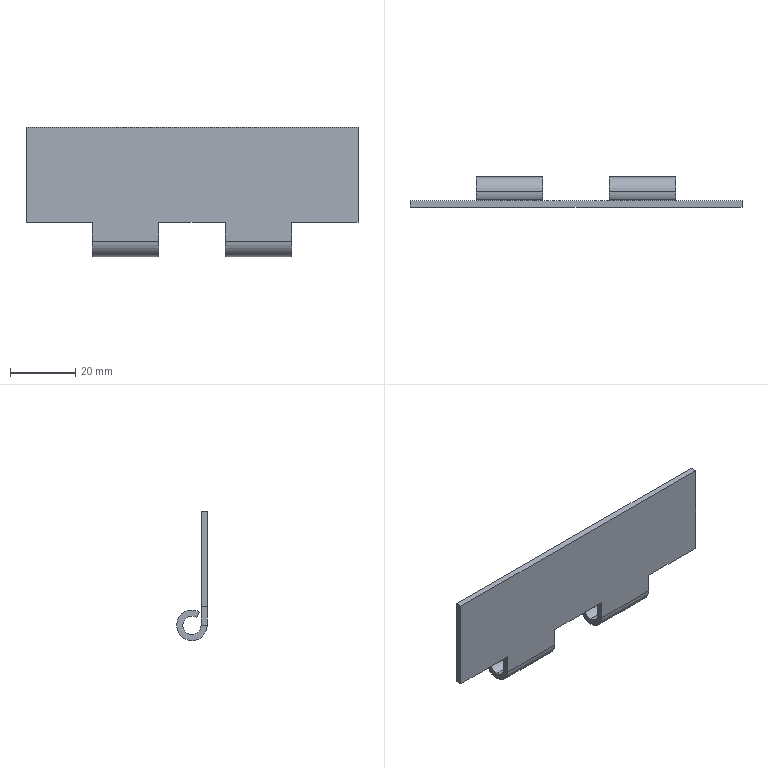Part | SolidWorks | features FlatPattern 1, ICE 1, SMBaseFlange 1, SheetMetal 1 | 1 solid | 28 faces | box 102 x 9.4 x 39.7 mm | volume 7631 mm3 | plane 16 | cylinder 12 | commonest cylinder face diameters 5.6 x6 9.4 x6
STEP:
#1=CARTESIAN_POINT('',(30.6,4.7,-37.8));
#2=VERTEX_POINT('',#1);
#3=CARTESIAN_POINT('',(30.6,1.9,-35.));
#4=VERTEX_POINT('',#3);
#5=CARTESIAN_POINT('',(30.6,4.7,-35.));
#6=DIRECTION('',(-1.,0.,0.));
#7=DIRECTION('',(0.,0.,1.));
#8=AXIS2_PLACEMENT_3D('',#5,#6,#7);
#9=CIRCLE('',#8,2.8);
#10=EDGE_CURVE('',#2,#4,#9,.T.);
#11=ORIENTED_EDGE('',*,*,#10,.F.);
#12=CARTESIAN_POINT('',(10.2,4.7,-37.8));
#13=VERTEX_POINT('',#12);
#14=CARTESIAN_POINT('',(51.,4.7,-37.8));
#15=DIRECTION('',(-1.,0.,0.));
#16=VECTOR('',#15,1000.);
#17=LINE('',#14,#16);
#18=EDGE_CURVE('',#2,#13,#17,.T.);
#19=ORIENTED_EDGE('',*,*,#18,.T.);
#20=CARTESIAN_POINT('',(10.2,1.9,-35.));
#21=VERTEX_POINT('',#20);
#22=CARTESIAN_POINT('',(10.2,4.7,-35.));
#23=DIRECTION('',(1.,0.,0.));
#24=DIRECTION('',(0.,0.,-1.));
#25=AXIS2_PLACEMENT_3D('',#22,#23,#24);
#26=CIRCLE('',#25,2.8);
#27=EDGE_CURVE('',#21,#13,#26,.T.);
#28=ORIENTED_EDGE('',*,*,#27,.F.);
#29=CARTESIAN_POINT('',(51.,1.9,-35.));
#30=DIRECTION('',(-1.,0.,0.));
#31=VECTOR('',#30,1000.);
#32=LINE('',#29,#31);
#33=EDGE_CURVE('',#4,#21,#32,.T.);
#34=ORIENTED_EDGE('',*,*,#33,.F.);
#35=EDGE_LOOP('',(#11,#19,#28,#34));
#36=FACE_OUTER_BOUND('',#35,.T.);
#37=CARTESIAN_POINT('',(51.,4.7,-35.));
#38=DIRECTION('',(-1.,0.,0.));
#39=DIRECTION('',(0.,0.,1.));
#40=AXIS2_PLACEMENT_3D('',#37,#38,#39);
#41=CYLINDRICAL_SURFACE('',#40,2.8);
#42=ADVANCED_FACE('',(#36),#41,.F.);
#43=ORIENTED_EDGE('',*,*,#18,.F.);
#44=CARTESIAN_POINT('',(30.6,4.7,-32.2));
#45=VERTEX_POINT('',#44);
#46=CARTESIAN_POINT('',(30.6,4.7,-35.));
#47=DIRECTION('',(-1.,0.,0.));
#48=DIRECTION('',(0.,0.,1.));
#49=AXIS2_PLACEMENT_3D('',#46,#47,#48);
#50=CIRCLE('',#49,2.8);
#51=EDGE_CURVE('',#45,#2,#50,.T.);
#52=ORIENTED_EDGE('',*,*,#51,.F.);
#53=CARTESIAN_POINT('',(10.2,4.7,-32.2));
#54=VERTEX_POINT('',#53);
#55=CARTESIAN_POINT('',(51.,4.7,-32.2));
#56=DIRECTION('',(-1.,0.,0.));
#57=VECTOR('',#56,1000.);
#58=LINE('',#55,#57);
#59=EDGE_CURVE('',#45,#54,#58,.T.);
#60=ORIENTED_EDGE('',*,*,#59,.T.);
#61=CARTESIAN_POINT('',(10.2,4.7,-35.));
#62=DIRECTION('',(1.,0.,0.));
#63=DIRECTION('',(0.,0.,-1.));
#64=AXIS2_PLACEMENT_3D('',#61,#62,#63);
#65=CIRCLE('',#64,2.8);
#66=EDGE_CURVE('',#13,#54,#65,.T.);
#67=ORIENTED_EDGE('',*,*,#66,.F.);
#68=EDGE_LOOP('',(#43,#52,#60,#67));
#69=FACE_OUTER_BOUND('',#68,.T.);
#70=CARTESIAN_POINT('',(51.,4.7,-35.));
#71=DIRECTION('',(-1.,0.,0.));
#72=DIRECTION('',(0.,0.,1.));
#73=AXIS2_PLACEMENT_3D('',#70,#71,#72);
#74=CYLINDRICAL_SURFACE('',#73,2.8);
#75=ADVANCED_FACE('',(#69),#74,.F.);
#76=CARTESIAN_POINT('',(30.6,4.7,-30.3));
#77=VERTEX_POINT('',#76);
#78=CARTESIAN_POINT('',(30.6,4.7,-39.7));
#79=VERTEX_POINT('',#78);
#80=CARTESIAN_POINT('',(30.6,4.7,-35.));
#81=DIRECTION('',(-1.,0.,0.));
#82=DIRECTION('',(0.,0.,1.));
#83=AXIS2_PLACEMENT_3D('',#80,#81,#82);
#84=CIRCLE('',#83,4.7);
#85=EDGE_CURVE('',#77,#79,#84,.T.);
#86=ORIENTED_EDGE('',*,*,#85,.T.);
#87=CARTESIAN_POINT('',(10.2,4.7,-39.7));
#88=VERTEX_POINT('',#87);
#89=CARTESIAN_POINT('',(51.,4.7,-39.7));
#90=DIRECTION('',(-1.,0.,0.));
#91=VECTOR('',#90,1000.);
#92=LINE('',#89,#91);
#93=EDGE_CURVE('',#79,#88,#92,.T.);
#94=ORIENTED_EDGE('',*,*,#93,.T.);
#95=CARTESIAN_POINT('',(10.2,4.7,-30.3));
#96=VERTEX_POINT('',#95);
#97=CARTESIAN_POINT('',(10.2,4.7,-35.));
#98=DIRECTION('',(1.,0.,0.));
#99=DIRECTION('',(0.,0.,-1.));
#100=AXIS2_PLACEMENT_3D('',#97,#98,#99);
#101=CIRCLE('',#100,4.7);
#102=EDGE_CURVE('',#88,#96,#101,.T.);
#103=ORIENTED_EDGE('',*,*,#102,.T.);
#104=CARTESIAN_POINT('',(51.,4.7,-30.3));
#105=DIRECTION('',(-1.,0.,0.));
#106=VECTOR('',#105,1000.);
#107=LINE('',#104,#106);
#108=EDGE_CURVE('',#77,#96,#107,.T.);
#109=ORIENTED_EDGE('',*,*,#108,.F.);
#110=EDGE_LOOP('',(#86,#94,#103,#109));
#111=FACE_OUTER_BOUND('',#110,.T.);
#112=CARTESIAN_POINT('',(51.,4.7,-35.));
#113=DIRECTION('',(-1.,0.,0.));
#114=DIRECTION('',(0.,0.,1.));
#115=AXIS2_PLACEMENT_3D('',#112,#113,#114);
#116=CYLINDRICAL_SURFACE('',#115,4.7);
#117=ADVANCED_FACE('',(#111),#116,.T.);
#118=CARTESIAN_POINT('',(30.6,2.35,-30.93));
#119=VERTEX_POINT('',#118);
#120=CARTESIAN_POINT('',(30.6,4.7,-35.));
#121=DIRECTION('',(-1.,0.,0.));
#122=DIRECTION('',(0.,0.,1.));
#123=AXIS2_PLACEMENT_3D('',#120,#121,#122);
#124=CIRCLE('',#123,4.7);
#125=EDGE_CURVE('',#119,#77,#124,.T.);
#126=ORIENTED_EDGE('',*,*,#125,.T.);
#127=ORIENTED_EDGE('',*,*,#108,.T.);
#128=CARTESIAN_POINT('',(10.2,2.35,-30.93));
#129=VERTEX_POINT('',#128);
#130=CARTESIAN_POINT('',(10.2,4.7,-35.));
#131=DIRECTION('',(1.,0.,0.));
#132=DIRECTION('',(0.,0.,-1.));
#133=AXIS2_PLACEMENT_3D('',#130,#131,#132);
#134=CIRCLE('',#133,4.7);
#135=EDGE_CURVE('',#96,#129,#134,.T.);
#136=ORIENTED_EDGE('',*,*,#135,.T.);
#137=CARTESIAN_POINT('',(51.,2.35,-30.93));
#138=DIRECTION('',(-1.,0.,0.));
#139=VECTOR('',#138,1000.);
#140=LINE('',#137,#139);
#141=EDGE_CURVE('',#119,#129,#140,.T.);
#142=ORIENTED_EDGE('',*,*,#141,.F.);
#143=EDGE_LOOP('',(#126,#127,#136,#142));
#144=FACE_OUTER_BOUND('',#143,.T.);
#145=CARTESIAN_POINT('',(51.,4.7,-35.));
#146=DIRECTION('',(-1.,0.,0.));
#147=DIRECTION('',(0.,0.,1.));
#148=AXIS2_PLACEMENT_3D('',#145,#146,#147);
#149=CYLINDRICAL_SURFACE('',#148,4.7);
#150=ADVANCED_FACE('',(#144),#149,.T.);
#151=CARTESIAN_POINT('',(-10.2,4.7,-37.8));
#152=VERTEX_POINT('',#151);
#153=CARTESIAN_POINT('',(-10.2,1.9,-35.));
#154=VERTEX_POINT('',#153);
#155=CARTESIAN_POINT('',(-10.2,4.7,-35.));
#156=DIRECTION('',(-1.,0.,0.));
#157=DIRECTION('',(0.,0.,1.));
#158=AXIS2_PLACEMENT_3D('',#155,#156,#157);
#159=CIRCLE('',#158,2.8);
#160=EDGE_CURVE('',#152,#154,#159,.T.);
#161=ORIENTED_EDGE('',*,*,#160,.F.);
#162=CARTESIAN_POINT('',(-30.6,4.7,-37.8));
#163=VERTEX_POINT('',#162);
#164=CARTESIAN_POINT('',(51.,4.7,-37.8));
#165=DIRECTION('',(-1.,0.,0.));
#166=VECTOR('',#165,1000.);
#167=LINE('',#164,#166);
#168=EDGE_CURVE('',#152,#163,#167,.T.);
#169=ORIENTED_EDGE('',*,*,#168,.T.);
#170=CARTESIAN_POINT('',(-30.6,1.9,-35.));
#171=VERTEX_POINT('',#170);
#172=CARTESIAN_POINT('',(-30.6,4.7,-35.));
#173=DIRECTION('',(1.,0.,0.));
#174=DIRECTION('',(0.,0.,-1.));
#175=AXIS2_PLACEMENT_3D('',#172,#173,#174);
#176=CIRCLE('',#175,2.8);
#177=EDGE_CURVE('',#171,#163,#176,.T.);
#178=ORIENTED_EDGE('',*,*,#177,.F.);
#179=CARTESIAN_POINT('',(51.,1.9,-35.));
#180=DIRECTION('',(-1.,0.,0.));
#181=VECTOR('',#180,1000.);
#182=LINE('',#179,#181);
#183=EDGE_CURVE('',#154,#171,#182,.T.);
#184=ORIENTED_EDGE('',*,*,#183,.F.);
#185=EDGE_LOOP('',(#161,#169,#178,#184));
#186=FACE_OUTER_BOUND('',#185,.T.);
#187=CARTESIAN_POINT('',(51.,4.7,-35.));
#188=DIRECTION('',(-1.,0.,0.));
#189=DIRECTION('',(0.,0.,1.));
#190=AXIS2_PLACEMENT_3D('',#187,#188,#189);
#191=CYLINDRICAL_SURFACE('',#190,2.8);
#192=ADVANCED_FACE('',(#186),#191,.F.);
#193=ORIENTED_EDGE('',*,*,#168,.F.);
#194=CARTESIAN_POINT('',(-10.2,4.7,-32.2));
#195=VERTEX_POINT('',#194);
#196=CARTESIAN_POINT('',(-10.2,4.7,-35.));
#197=DIRECTION('',(-1.,0.,0.));
#198=DIRECTION('',(0.,0.,1.));
#199=AXIS2_PLACEMENT_3D('',#196,#197,#198);
#200=CIRCLE('',#199,2.8);
#201=EDGE_CURVE('',#195,#152,#200,.T.);
#202=ORIENTED_EDGE('',*,*,#201,.F.);
#203=CARTESIAN_POINT('',(-30.6,4.7,-32.2));
#204=VERTEX_POINT('',#203);
#205=CARTESIAN_POINT('',(51.,4.7,-32.2));
#206=DIRECTION('',(-1.,0.,0.));
#207=VECTOR('',#206,1000.);
#208=LINE('',#205,#207);
#209=EDGE_CURVE('',#195,#204,#208,.T.);
#210=ORIENTED_EDGE('',*,*,#209,.T.);
#211=CARTESIAN_POINT('',(-30.6,4.7,-35.));
#212=DIRECTION('',(1.,0.,0.));
#213=DIRECTION('',(0.,0.,-1.));
#214=AXIS2_PLACEMENT_3D('',#211,#212,#213);
#215=CIRCLE('',#214,2.8);
#216=EDGE_CURVE('',#163,#204,#215,.T.);
#217=ORIENTED_EDGE('',*,*,#216,.F.);
#218=EDGE_LOOP('',(#193,#202,#210,#217));
#219=FACE_OUTER_BOUND('',#218,.T.);
#220=CARTESIAN_POINT('',(51.,4.7,-35.));
#221=DIRECTION('',(-1.,0.,0.));
#222=DIRECTION('',(0.,0.,1.));
#223=AXIS2_PLACEMENT_3D('',#220,#221,#222);
#224=CYLINDRICAL_SURFACE('',#223,2.8);
#225=ADVANCED_FACE('',(#219),#224,.F.);
#226=CARTESIAN_POINT('',(-10.2,4.7,-30.3));
#227=VERTEX_POINT('',#226);
#228=CARTESIAN_POINT('',(-10.2,4.7,-39.7));
#229=VERTEX_POINT('',#228);
#230=CARTESIAN_POINT('',(-10.2,4.7,-35.));
#231=DIRECTION('',(-1.,0.,0.));
#232=DIRECTION('',(0.,0.,1.));
#233=AXIS2_PLACEMENT_3D('',#230,#231,#232);
#234=CIRCLE('',#233,4.7);
#235=EDGE_CURVE('',#227,#229,#234,.T.);
#236=ORIENTED_EDGE('',*,*,#235,.T.);
#237=CARTESIAN_POINT('',(-30.6,4.7,-39.7));
#238=VERTEX_POINT('',#237);
#239=CARTESIAN_POINT('',(51.,4.7,-39.7));
#240=DIRECTION('',(-1.,0.,0.));
#241=VECTOR('',#240,1000.);
#242=LINE('',#239,#241);
#243=EDGE_CURVE('',#229,#238,#242,.T.);
#244=ORIENTED_EDGE('',*,*,#243,.T.);
#245=CARTESIAN_POINT('',(-30.6,4.7,-30.3));
#246=VERTEX_POINT('',#245);
#247=CARTESIAN_POINT('',(-30.6,4.7,-35.));
#248=DIRECTION('',(1.,0.,0.));
#249=DIRECTION('',(0.,0.,-1.));
#250=AXIS2_PLACEMENT_3D('',#247,#248,#249);
#251=CIRCLE('',#250,4.7);
#252=EDGE_CURVE('',#238,#246,#251,.T.);
#253=ORIENTED_EDGE('',*,*,#252,.T.);
#254=CARTESIAN_POINT('',(51.,4.7,-30.3));
#255=DIRECTION('',(-1.,0.,0.));
#256=VECTOR('',#255,1000.);
#257=LINE('',#254,#256);
#258=EDGE_CURVE('',#227,#246,#257,.T.);
#259=ORIENTED_EDGE('',*,*,#258,.F.);
#260=EDGE_LOOP('',(#236,#244,#253,#259));
#261=FACE_OUTER_BOUND('',#260,.T.);
#262=CARTESIAN_POINT('',(51.,4.7,-35.));
#263=DIRECTION('',(-1.,0.,0.));
#264=DIRECTION('',(0.,0.,1.));
#265=AXIS2_PLACEMENT_3D('',#262,#263,#264);
#266=CYLINDRICAL_SURFACE('',#265,4.7);
#267=ADVANCED_FACE('',(#261),#266,.T.);
#268=CARTESIAN_POINT('',(-10.2,2.35,-30.93));
#269=VERTEX_POINT('',#268);
#270=CARTESIAN_POINT('',(-10.2,4.7,-35.));
#271=DIRECTION('',(-1.,0.,0.));
#272=DIRECTION('',(0.,0.,1.));
#273=AXIS2_PLACEMENT_3D('',#270,#271,#272);
#274=CIRCLE('',#273,4.7);
#275=EDGE_CURVE('',#269,#227,#274,.T.);
#276=ORIENTED_EDGE('',*,*,#275,.T.);
#277=ORIENTED_EDGE('',*,*,#258,.T.);
#278=CARTESIAN_POINT('',(-30.6,2.35,-30.93));
#279=VERTEX_POINT('',#278);
#280=CARTESIAN_POINT('',(-30.6,4.7,-35.));
#281=DIRECTION('',(1.,0.,0.));
#282=DIRECTION('',(0.,0.,-1.));
#283=AXIS2_PLACEMENT_3D('',#280,#281,#282);
#284=CIRCLE('',#283,4.7);
#285=EDGE_CURVE('',#246,#279,#284,.T.);
#286=ORIENTED_EDGE('',*,*,#285,.T.);
#287=CARTESIAN_POINT('',(51.,2.35,-30.93));
#288=DIRECTION('',(-1.,0.,0.));
#289=VECTOR('',#288,1000.);
#290=LINE('',#287,#289);
#291=EDGE_CURVE('',#269,#279,#290,.T.);
#292=ORIENTED_EDGE('',*,*,#291,.F.);
#293=EDGE_LOOP('',(#276,#277,#286,#292));
#294=FACE_OUTER_BOUND('',#293,.T.);
#295=CARTESIAN_POINT('',(51.,4.7,-35.));
#296=DIRECTION('',(-1.,0.,0.));
#297=DIRECTION('',(0.,0.,1.));
#298=AXIS2_PLACEMENT_3D('',#295,#296,#297);
#299=CYLINDRICAL_SURFACE('',#298,4.7);
#300=ADVANCED_FACE('',(#294),#299,.T.);
#301=CARTESIAN_POINT('',(10.2,1.9,-29.2));
#302=VERTEX_POINT('',#301);
#303=CARTESIAN_POINT('',(10.2,1.9,0.));
#304=DIRECTION('',(0.,0.,-1.));
#305=VECTOR('',#304,1000.);
#306=LINE('',#303,#305);
#307=EDGE_CURVE('',#302,#21,#306,.T.);
#308=ORIENTED_EDGE('',*,*,#307,.T.);
#309=CARTESIAN_POINT('',(10.2,0.,-35.));
#310=VERTEX_POINT('',#309);
#311=CARTESIAN_POINT('',(10.2,1.9,-35.));
#312=DIRECTION('',(0.,-1.,0.));
#313=VECTOR('',#312,1000.);
#314=LINE('',#311,#313);
#315=EDGE_CURVE('',#21,#310,#314,.T.);
#316=ORIENTED_EDGE('',*,*,#315,.T.);
#317=CARTESIAN_POINT('',(10.2,0.,-29.2));
#318=VERTEX_POINT('',#317);
#319=CARTESIAN_POINT('',(10.2,0.,0.));
#320=DIRECTION('',(0.,0.,-1.));
#321=VECTOR('',#320,1000.);
#322=LINE('',#319,#321);
#323=EDGE_CURVE('',#318,#310,#322,.T.);
#324=ORIENTED_EDGE('',*,*,#323,.F.);
#325=CARTESIAN_POINT('',(10.2,9.4,-29.2));
#326=DIRECTION('',(0.,-1.,0.));
#327=VECTOR('',#326,1000.);
#328=LINE('',#325,#327);
#329=EDGE_CURVE('',#302,#318,#328,.T.);
#330=ORIENTED_EDGE('',*,*,#329,.F.);
#331=EDGE_LOOP('',(#308,#316,#324,#330));
#332=FACE_OUTER_BOUND('',#331,.T.);
#333=CARTESIAN_POINT('',(10.2,9.4,-39.7));
#334=DIRECTION('',(1.,0.,0.));
#335=DIRECTION('',(0.,0.,-1.));
#336=AXIS2_PLACEMENT_3D('',#333,#334,#335);
#337=PLANE('',#336);
#338=ADVANCED_FACE('',(#332),#337,.F.);
#339=CARTESIAN_POINT('',(-30.6,1.9,-29.2));
#340=VERTEX_POINT('',#339);
#341=CARTESIAN_POINT('',(-30.6,1.9,0.));
#342=DIRECTION('',(0.,0.,-1.));
#343=VECTOR('',#342,1000.);
#344=LINE('',#341,#343);
#345=EDGE_CURVE('',#340,#171,#344,.T.);
#346=ORIENTED_EDGE('',*,*,#345,.T.);
#347=CARTESIAN_POINT('',(-30.6,0.,-35.));
#348=VERTEX_POINT('',#347);
#349=CARTESIAN_POINT('',(-30.6,1.9,-35.));
#350=DIRECTION('',(0.,-1.,0.));
#351=VECTOR('',#350,1000.);
#352=LINE('',#349,#351);
#353=EDGE_CURVE('',#171,#348,#352,.T.);
#354=ORIENTED_EDGE('',*,*,#353,.T.);
#355=CARTESIAN_POINT('',(-30.6,0.,-29.2));
#356=VERTEX_POINT('',#355);
#357=CARTESIAN_POINT('',(-30.6,0.,-39.7));
#358=DIRECTION('',(0.,0.,1.));
#359=VECTOR('',#358,1000.);
#360=LINE('',#357,#359);
#361=EDGE_CURVE('',#348,#356,#360,.T.);
#362=ORIENTED_EDGE('',*,*,#361,.T.);
#363=CARTESIAN_POINT('',(-30.6,9.4,-29.2));
#364=DIRECTION('',(0.,-1.,0.));
#365=VECTOR('',#364,1000.);
#366=LINE('',#363,#365);
#367=EDGE_CURVE('',#340,#356,#366,.T.);
#368=ORIENTED_EDGE('',*,*,#367,.F.);
#369=EDGE_LOOP('',(#346,#354,#362,#368));
#370=FACE_OUTER_BOUND('',#369,.T.);
#371=CARTESIAN_POINT('',(-30.6,9.4,-39.7));
#372=DIRECTION('',(1.,0.,0.));
#373=DIRECTION('',(0.,0.,-1.));
#374=AXIS2_PLACEMENT_3D('',#371,#372,#373);
#375=PLANE('',#374);
#376=ADVANCED_FACE('',(#370),#375,.F.);
#377=ORIENTED_EDGE('',*,*,#243,.F.);
#378=CARTESIAN_POINT('',(-10.2,0.,-35.));
#379=VERTEX_POINT('',#378);
#380=CARTESIAN_POINT('',(-10.2,4.7,-35.));
#381=DIRECTION('',(-1.,0.,0.));
#382=DIRECTION('',(0.,0.,1.));
#383=AXIS2_PLACEMENT_3D('',#380,#381,#382);
#384=CIRCLE('',#383,4.7);
#385=EDGE_CURVE('',#229,#379,#384,.T.);
#386=ORIENTED_EDGE('',*,*,#385,.T.);
#387=CARTESIAN_POINT('',(51.,0.,-35.));
#388=DIRECTION('',(-1.,0.,0.));
#389=VECTOR('',#388,1000.);
#390=LINE('',#387,#389);
#391=EDGE_CURVE('',#379,#348,#390,.T.);
#392=ORIENTED_EDGE('',*,*,#391,.T.);
#393=CARTESIAN_POINT('',(-30.6,4.7,-35.));
#394=DIRECTION('',(1.,0.,0.));
#395=DIRECTION('',(0.,0.,-1.));
#396=AXIS2_PLACEMENT_3D('',#393,#394,#395);
#397=CIRCLE('',#396,4.7);
#398=EDGE_CURVE('',#348,#238,#397,.T.);
#399=ORIENTED_EDGE('',*,*,#398,.T.);
#400=EDGE_LOOP('',(#377,#386,#392,#399));
#401=FACE_OUTER_BOUND('',#400,.T.);
#402=CARTESIAN_POINT('',(51.,4.7,-35.));
#403=DIRECTION('',(-1.,0.,0.));
#404=DIRECTION('',(0.,0.,1.));
#405=AXIS2_PLACEMENT_3D('',#402,#403,#404);
#406=CYLINDRICAL_SURFACE('',#405,4.7);
#407=ADVANCED_FACE('',(#401),#406,.T.);
#408=CARTESIAN_POINT('',(-30.6,3.3,-32.575));
#409=VERTEX_POINT('',#408);
#410=CARTESIAN_POINT('',(-30.6,3.3,-32.575));
#411=DIRECTION('',(0.,-0.5,0.866));
#412=VECTOR('',#411,1000.);
#413=LINE('',#410,#412);
#414=EDGE_CURVE('',#409,#279,#413,.T.);
#415=ORIENTED_EDGE('',*,*,#414,.F.);
#416=CARTESIAN_POINT('',(-10.2,3.3,-32.575));
#417=VERTEX_POINT('',#416);
#418=CARTESIAN_POINT('',(51.,3.3,-32.575));
#419=DIRECTION('',(-1.,0.,0.));
#420=VECTOR('',#419,1000.);
#421=LINE('',#418,#420);
#422=EDGE_CURVE('',#417,#409,#421,.T.);
#423=ORIENTED_EDGE('',*,*,#422,.F.);
#424=CARTESIAN_POINT('',(-10.2,3.3,-32.575));
#425=DIRECTION('',(0.,0.5,-0.866));
#426=VECTOR('',#425,1000.);
#427=LINE('',#424,#426);
#428=EDGE_CURVE('',#269,#417,#427,.T.);
#429=ORIENTED_EDGE('',*,*,#428,.F.);
#430=ORIENTED_EDGE('',*,*,#291,.T.);
#431=EDGE_LOOP('',(#415,#423,#429,#430));
#432=FACE_OUTER_BOUND('',#431,.T.);
#433=CARTESIAN_POINT('',(51.,3.3,-32.575));
#434=DIRECTION('',(0.,-0.866,-0.5));
#435=DIRECTION('',(0.,0.5,-0.866));
#436=AXIS2_PLACEMENT_3D('',#433,#434,#435);
#437=PLANE('',#436);
#438=ADVANCED_FACE('',(#432),#437,.T.);
#439=ORIENTED_EDGE('',*,*,#209,.F.);
#440=CARTESIAN_POINT('',(-10.2,4.7,-35.));
#441=DIRECTION('',(-1.,0.,0.));
#442=DIRECTION('',(0.,0.,1.));
#443=AXIS2_PLACEMENT_3D('',#440,#441,#442);
#444=CIRCLE('',#443,2.8);
#445=EDGE_CURVE('',#417,#195,#444,.T.);
#446=ORIENTED_EDGE('',*,*,#445,.F.);
#447=ORIENTED_EDGE('',*,*,#422,.T.);
#448=CARTESIAN_POINT('',(-30.6,4.7,-35.));
#449=DIRECTION('',(1.,0.,0.));
#450=DIRECTION('',(0.,0.,-1.));
#451=AXIS2_PLACEMENT_3D('',#448,#449,#450);
#452=CIRCLE('',#451,2.8);
#453=EDGE_CURVE('',#204,#409,#452,.T.);
#454=ORIENTED_EDGE('',*,*,#453,.F.);
#455=EDGE_LOOP('',(#439,#446,#447,#454));
#456=FACE_OUTER_BOUND('',#455,.T.);
#457=CARTESIAN_POINT('',(51.,4.7,-35.));
#458=DIRECTION('',(-1.,0.,0.));
#459=DIRECTION('',(0.,0.,1.));
#460=AXIS2_PLACEMENT_3D('',#457,#458,#459);
#461=CYLINDRICAL_SURFACE('',#460,2.8);
#462=ADVANCED_FACE('',(#456),#461,.F.);
#463=ORIENTED_EDGE('',*,*,#93,.F.);
#464=CARTESIAN_POINT('',(30.6,0.,-35.));
#465=VERTEX_POINT('',#464);
#466=CARTESIAN_POINT('',(30.6,4.7,-35.));
#467=DIRECTION('',(-1.,0.,0.));
#468=DIRECTION('',(0.,0.,1.));
#469=AXIS2_PLACEMENT_3D('',#466,#467,#468);
#470=CIRCLE('',#469,4.7);
#471=EDGE_CURVE('',#79,#465,#470,.T.);
#472=ORIENTED_EDGE('',*,*,#471,.T.);
#473=CARTESIAN_POINT('',(51.,0.,-35.));
#474=DIRECTION('',(-1.,0.,0.));
#475=VECTOR('',#474,1000.);
#476=LINE('',#473,#475);
#477=EDGE_CURVE('',#465,#310,#476,.T.);
#478=ORIENTED_EDGE('',*,*,#477,.T.);
#479=CARTESIAN_POINT('',(10.2,4.7,-35.));
#480=DIRECTION('',(1.,0.,0.));
#481=DIRECTION('',(0.,0.,-1.));
#482=AXIS2_PLACEMENT_3D('',#479,#480,#481);
#483=CIRCLE('',#482,4.7);
#484=EDGE_CURVE('',#310,#88,#483,.T.);
#485=ORIENTED_EDGE('',*,*,#484,.T.);
#486=EDGE_LOOP('',(#463,#472,#478,#485));
#487=FACE_OUTER_BOUND('',#486,.T.);
#488=CARTESIAN_POINT('',(51.,4.7,-35.));
#489=DIRECTION('',(-1.,0.,0.));
#490=DIRECTION('',(0.,0.,1.));
#491=AXIS2_PLACEMENT_3D('',#488,#489,#490);
#492=CYLINDRICAL_SURFACE('',#491,4.7);
#493=ADVANCED_FACE('',(#487),#492,.T.);
#494=CARTESIAN_POINT('',(10.2,3.3,-32.575));
#495=VERTEX_POINT('',#494);
#496=CARTESIAN_POINT('',(10.2,3.3,-32.575));
#497=DIRECTION('',(0.,-0.5,0.866));
#498=VECTOR('',#497,1000.);
#499=LINE('',#496,#498);
#500=EDGE_CURVE('',#495,#129,#499,.T.);
#501=ORIENTED_EDGE('',*,*,#500,.F.);
#502=CARTESIAN_POINT('',(30.6,3.3,-32.575));
#503=VERTEX_POINT('',#502);
#504=CARTESIAN_POINT('',(51.,3.3,-32.575));
#505=DIRECTION('',(-1.,0.,0.));
#506=VECTOR('',#505,1000.);
#507=LINE('',#504,#506);
#508=EDGE_CURVE('',#503,#495,#507,.T.);
#509=ORIENTED_EDGE('',*,*,#508,.F.);
#510=CARTESIAN_POINT('',(30.6,3.3,-32.575));
#511=DIRECTION('',(0.,0.5,-0.866));
#512=VECTOR('',#511,1000.);
#513=LINE('',#510,#512);
#514=EDGE_CURVE('',#119,#503,#513,.T.);
#515=ORIENTED_EDGE('',*,*,#514,.F.);
#516=ORIENTED_EDGE('',*,*,#141,.T.);
#517=EDGE_LOOP('',(#501,#509,#515,#516));
#518=FACE_OUTER_BOUND('',#517,.T.);
#519=CARTESIAN_POINT('',(51.,3.3,-32.575));
#520=DIRECTION('',(0.,-0.866,-0.5));
#521=DIRECTION('',(0.,0.5,-0.866));
#522=AXIS2_PLACEMENT_3D('',#519,#520,#521);
#523=PLANE('',#522);
#524=ADVANCED_FACE('',(#518),#523,.T.);
#525=ORIENTED_EDGE('',*,*,#59,.F.);
#526=CARTESIAN_POINT('',(30.6,4.7,-35.));
#527=DIRECTION('',(-1.,0.,0.));
#528=DIRECTION('',(0.,0.,1.));
#529=AXIS2_PLACEMENT_3D('',#526,#527,#528);
#530=CIRCLE('',#529,2.8);
#531=EDGE_CURVE('',#503,#45,#530,.T.);
#532=ORIENTED_EDGE('',*,*,#531,.F.);
#533=ORIENTED_EDGE('',*,*,#508,.T.);
#534=CARTESIAN_POINT('',(10.2,4.7,-35.));
#535=DIRECTION('',(1.,0.,0.));
#536=DIRECTION('',(0.,0.,-1.));
#537=AXIS2_PLACEMENT_3D('',#534,#535,#536);
#538=CIRCLE('',#537,2.8);
#539=EDGE_CURVE('',#54,#495,#538,.T.);
#540=ORIENTED_EDGE('',*,*,#539,.F.);
#541=EDGE_LOOP('',(#525,#532,#533,#540));
#542=FACE_OUTER_BOUND('',#541,.T.);
#543=CARTESIAN_POINT('',(51.,4.7,-35.));
#544=DIRECTION('',(-1.,0.,0.));
#545=DIRECTION('',(0.,0.,1.));
#546=AXIS2_PLACEMENT_3D('',#543,#544,#545);
#547=CYLINDRICAL_SURFACE('',#546,2.8);
#548=ADVANCED_FACE('',(#542),#547,.F.);
#549=CARTESIAN_POINT('',(-51.,1.9,-29.2));
#550=VERTEX_POINT('',#549);
#551=CARTESIAN_POINT('',(51.,1.9,-29.2));
#552=DIRECTION('',(1.,0.,0.));
#553=VECTOR('',#552,1000.);
#554=LINE('',#551,#553);
#555=EDGE_CURVE('',#550,#340,#554,.T.);
#556=ORIENTED_EDGE('',*,*,#555,.F.);
#557=CARTESIAN_POINT('',(-51.,1.9,0.));
#558=VERTEX_POINT('',#557);
#559=CARTESIAN_POINT('',(-51.,1.9,0.));
#560=DIRECTION('',(0.,0.,-1.));
#561=VECTOR('',#560,1000.);
#562=LINE('',#559,#561);
#563=EDGE_CURVE('',#558,#550,#562,.T.);
#564=ORIENTED_EDGE('',*,*,#563,.F.);
#565=CARTESIAN_POINT('',(51.,1.9,0.));
#566=VERTEX_POINT('',#565);
#567=CARTESIAN_POINT('',(51.,1.9,0.));
#568=DIRECTION('',(-1.,0.,0.));
#569=VECTOR('',#568,1000.);
#570=LINE('',#567,#569);
#571=EDGE_CURVE('',#566,#558,#570,.T.);
#572=ORIENTED_EDGE('',*,*,#571,.F.);
#573=CARTESIAN_POINT('',(51.,1.9,-29.2));
#574=VERTEX_POINT('',#573);
#575=CARTESIAN_POINT('',(51.,1.9,0.));
#576=DIRECTION('',(0.,0.,-1.));
#577=VECTOR('',#576,1000.);
#578=LINE('',#575,#577);
#579=EDGE_CURVE('',#566,#574,#578,.T.);
#580=ORIENTED_EDGE('',*,*,#579,.T.);
#581=CARTESIAN_POINT('',(30.6,1.9,-29.2));
#582=VERTEX_POINT('',#581);
#583=CARTESIAN_POINT('',(51.,1.9,-29.2));
#584=DIRECTION('',(1.,0.,0.));
#585=VECTOR('',#584,1000.);
#586=LINE('',#583,#585);
#587=EDGE_CURVE('',#582,#574,#586,.T.);
#588=ORIENTED_EDGE('',*,*,#587,.F.);
#589=CARTESIAN_POINT('',(30.6,1.9,0.));
#590=DIRECTION('',(0.,0.,1.));
#591=VECTOR('',#590,1000.);
#592=LINE('',#589,#591);
#593=EDGE_CURVE('',#4,#582,#592,.T.);
#594=ORIENTED_EDGE('',*,*,#593,.F.);
#595=ORIENTED_EDGE('',*,*,#33,.T.);
#596=ORIENTED_EDGE('',*,*,#307,.F.);
#597=CARTESIAN_POINT('',(-10.2,1.9,-29.2));
#598=VERTEX_POINT('',#597);
#599=CARTESIAN_POINT('',(51.,1.9,-29.2));
#600=DIRECTION('',(1.,0.,0.));
#601=VECTOR('',#600,1000.);
#602=LINE('',#599,#601);
#603=EDGE_CURVE('',#598,#302,#602,.T.);
#604=ORIENTED_EDGE('',*,*,#603,.F.);
#605=CARTESIAN_POINT('',(-10.2,1.9,0.));
#606=DIRECTION('',(0.,0.,1.));
#607=VECTOR('',#606,1000.);
#608=LINE('',#605,#607);
#609=EDGE_CURVE('',#154,#598,#608,.T.);
#610=ORIENTED_EDGE('',*,*,#609,.F.);
#611=ORIENTED_EDGE('',*,*,#183,.T.);
#612=ORIENTED_EDGE('',*,*,#345,.F.);
#613=EDGE_LOOP('',(#556,#564,#572,#580,#588,#594,#595,#596,#604,#610,#611,#612));
#614=FACE_OUTER_BOUND('',#613,.T.);
#615=CARTESIAN_POINT('',(51.,1.9,0.));
#616=DIRECTION('',(0.,1.,0.));
#617=DIRECTION('',(0.,0.,1.));
#618=AXIS2_PLACEMENT_3D('',#615,#616,#617);
#619=PLANE('',#618);
#620=ADVANCED_FACE('',(#614),#619,.T.);
#621=CARTESIAN_POINT('',(-51.,0.,0.));
#622=VERTEX_POINT('',#621);
#623=CARTESIAN_POINT('',(-51.,0.,0.));
#624=DIRECTION('',(0.,1.,0.));
#625=VECTOR('',#624,1000.);
#626=LINE('',#623,#625);
#627=EDGE_CURVE('',#622,#558,#626,.T.);
#628=ORIENTED_EDGE('',*,*,#627,.F.);
#629=CARTESIAN_POINT('',(51.,0.,0.));
#630=VERTEX_POINT('',#629);
#631=CARTESIAN_POINT('',(51.,0.,0.));
#632=DIRECTION('',(-1.,0.,0.));
#633=VECTOR('',#632,1000.);
#634=LINE('',#631,#633);
#635=EDGE_CURVE('',#630,#622,#634,.T.);
#636=ORIENTED_EDGE('',*,*,#635,.F.);
#637=CARTESIAN_POINT('',(51.,0.,0.));
#638=DIRECTION('',(0.,1.,0.));
#639=VECTOR('',#638,1000.);
#640=LINE('',#637,#639);
#641=EDGE_CURVE('',#630,#566,#640,.T.);
#642=ORIENTED_EDGE('',*,*,#641,.T.);
#643=ORIENTED_EDGE('',*,*,#571,.T.);
#644=EDGE_LOOP('',(#628,#636,#642,#643));
#645=FACE_OUTER_BOUND('',#644,.T.);
#646=CARTESIAN_POINT('',(51.,0.,0.));
#647=DIRECTION('',(0.,0.,1.));
#648=DIRECTION('',(1.,0.,0.));
#649=AXIS2_PLACEMENT_3D('',#646,#647,#648);
#650=PLANE('',#649);
#651=ADVANCED_FACE('',(#645),#650,.T.);
#652=CARTESIAN_POINT('',(-51.,0.,-29.2));
#653=VERTEX_POINT('',#652);
#654=CARTESIAN_POINT('',(-51.,0.,0.));
#655=DIRECTION('',(0.,0.,-1.));
#656=VECTOR('',#655,1000.);
#657=LINE('',#654,#656);
#658=EDGE_CURVE('',#622,#653,#657,.T.);
#659=ORIENTED_EDGE('',*,*,#658,.T.);
#660=CARTESIAN_POINT('',(-51.,0.,-29.2));
#661=DIRECTION('',(-1.,0.,0.));
#662=VECTOR('',#661,1000.);
#663=LINE('',#660,#662);
#664=EDGE_CURVE('',#356,#653,#663,.T.);
#665=ORIENTED_EDGE('',*,*,#664,.F.);
#666=ORIENTED_EDGE('',*,*,#361,.F.);
#667=ORIENTED_EDGE('',*,*,#391,.F.);
#668=CARTESIAN_POINT('',(-10.2,0.,-29.2));
#669=VERTEX_POINT('',#668);
#670=CARTESIAN_POINT('',(-10.2,0.,-39.7));
#671=DIRECTION('',(0.,0.,-1.));
#672=VECTOR('',#671,1000.);
#673=LINE('',#670,#672);
#674=EDGE_CURVE('',#669,#379,#673,.T.);
#675=ORIENTED_EDGE('',*,*,#674,.F.);
#676=CARTESIAN_POINT('',(-10.2,0.,-29.2));
#677=DIRECTION('',(-1.,0.,0.));
#678=VECTOR('',#677,1000.);
#679=LINE('',#676,#678);
#680=EDGE_CURVE('',#318,#669,#679,.T.);
#681=ORIENTED_EDGE('',*,*,#680,.F.);
#682=ORIENTED_EDGE('',*,*,#323,.T.);
#683=ORIENTED_EDGE('',*,*,#477,.F.);
#684=CARTESIAN_POINT('',(30.6,0.,-29.2));
#685=VERTEX_POINT('',#684);
#686=CARTESIAN_POINT('',(30.6,0.,-39.7));
#687=DIRECTION('',(0.,0.,-1.));
#688=VECTOR('',#687,1000.);
#689=LINE('',#686,#688);
#690=EDGE_CURVE('',#685,#465,#689,.T.);
#691=ORIENTED_EDGE('',*,*,#690,.F.);
#692=CARTESIAN_POINT('',(51.,0.,-29.2));
#693=VERTEX_POINT('',#692);
#694=CARTESIAN_POINT('',(51.,0.,-29.2));
#695=DIRECTION('',(-1.,0.,0.));
#696=VECTOR('',#695,1000.);
#697=LINE('',#694,#696);
#698=EDGE_CURVE('',#693,#685,#697,.T.);
#699=ORIENTED_EDGE('',*,*,#698,.F.);
#700=CARTESIAN_POINT('',(51.,0.,0.));
#701=DIRECTION('',(0.,0.,-1.));
#702=VECTOR('',#701,1000.);
#703=LINE('',#700,#702);
#704=EDGE_CURVE('',#630,#693,#703,.T.);
#705=ORIENTED_EDGE('',*,*,#704,.F.);
#706=ORIENTED_EDGE('',*,*,#635,.T.);
#707=EDGE_LOOP('',(#659,#665,#666,#667,#675,#681,#682,#683,#691,#699,#705,#706));
#708=FACE_OUTER_BOUND('',#707,.T.);
#709=CARTESIAN_POINT('',(51.,0.,0.));
#710=DIRECTION('',(0.,1.,0.));
#711=DIRECTION('',(0.,0.,1.));
#712=AXIS2_PLACEMENT_3D('',#709,#710,#711);
#713=PLANE('',#712);
#714=ADVANCED_FACE('',(#708),#713,.F.);
#715=CARTESIAN_POINT('',(51.,4.7,-29.2));
#716=DIRECTION('',(0.,-1.,0.));
#717=VECTOR('',#716,1000.);
#718=LINE('',#715,#717);
#719=EDGE_CURVE('',#574,#693,#718,.T.);
#720=ORIENTED_EDGE('',*,*,#719,.F.);
#721=ORIENTED_EDGE('',*,*,#579,.F.);
#722=ORIENTED_EDGE('',*,*,#641,.F.);
#723=ORIENTED_EDGE('',*,*,#704,.T.);
#724=EDGE_LOOP('',(#720,#721,#722,#723));
#725=FACE_OUTER_BOUND('',#724,.T.);
#726=CARTESIAN_POINT('',(51.,4.7,-35.));
#727=DIRECTION('',(1.,0.,0.));
#728=DIRECTION('',(0.,0.,-1.));
#729=AXIS2_PLACEMENT_3D('',#726,#727,#728);
#730=PLANE('',#729);
#731=ADVANCED_FACE('',(#725),#730,.T.);
#732=ORIENTED_EDGE('',*,*,#563,.T.);
#733=CARTESIAN_POINT('',(-51.,4.7,-29.2));
#734=DIRECTION('',(0.,-1.,0.));
#735=VECTOR('',#734,1000.);
#736=LINE('',#733,#735);
#737=EDGE_CURVE('',#550,#653,#736,.T.);
#738=ORIENTED_EDGE('',*,*,#737,.T.);
#739=ORIENTED_EDGE('',*,*,#658,.F.);
#740=ORIENTED_EDGE('',*,*,#627,.T.);
#741=EDGE_LOOP('',(#732,#738,#739,#740));
#742=FACE_OUTER_BOUND('',#741,.T.);
#743=CARTESIAN_POINT('',(-51.,4.7,-35.));
#744=DIRECTION('',(1.,0.,0.));
#745=DIRECTION('',(0.,0.,-1.));
#746=AXIS2_PLACEMENT_3D('',#743,#744,#745);
#747=PLANE('',#746);
#748=ADVANCED_FACE('',(#742),#747,.F.);
#749=ORIENTED_EDGE('',*,*,#353,.F.);
#750=ORIENTED_EDGE('',*,*,#177,.T.);
#751=ORIENTED_EDGE('',*,*,#216,.T.);
#752=ORIENTED_EDGE('',*,*,#453,.T.);
#753=ORIENTED_EDGE('',*,*,#414,.T.);
#754=ORIENTED_EDGE('',*,*,#285,.F.);
#755=ORIENTED_EDGE('',*,*,#252,.F.);
#756=ORIENTED_EDGE('',*,*,#398,.F.);
#757=EDGE_LOOP('',(#749,#750,#751,#752,#753,#754,#755,#756));
#758=FACE_OUTER_BOUND('',#757,.T.);
#759=CARTESIAN_POINT('',(-30.6,9.4,-39.7));
#760=DIRECTION('',(1.,0.,0.));
#761=DIRECTION('',(0.,0.,-1.));
#762=AXIS2_PLACEMENT_3D('',#759,#760,#761);
#763=PLANE('',#762);
#764=ADVANCED_FACE('',(#758),#763,.F.);
#765=ORIENTED_EDGE('',*,*,#555,.T.);
#766=ORIENTED_EDGE('',*,*,#367,.T.);
#767=ORIENTED_EDGE('',*,*,#664,.T.);
#768=ORIENTED_EDGE('',*,*,#737,.F.);
#769=EDGE_LOOP('',(#765,#766,#767,#768));
#770=FACE_OUTER_BOUND('',#769,.T.);
#771=CARTESIAN_POINT('',(-51.,9.4,-29.2));
#772=DIRECTION('',(0.,0.,1.));
#773=DIRECTION('',(1.,0.,0.));
#774=AXIS2_PLACEMENT_3D('',#771,#772,#773);
#775=PLANE('',#774);
#776=ADVANCED_FACE('',(#770),#775,.F.);
#777=ORIENTED_EDGE('',*,*,#125,.F.);
#778=ORIENTED_EDGE('',*,*,#514,.T.);
#779=ORIENTED_EDGE('',*,*,#531,.T.);
#780=ORIENTED_EDGE('',*,*,#51,.T.);
#781=ORIENTED_EDGE('',*,*,#10,.T.);
#782=ORIENTED_EDGE('',*,*,#593,.T.);
#783=CARTESIAN_POINT('',(30.6,9.4,-29.2));
#784=DIRECTION('',(0.,-1.,0.));
#785=VECTOR('',#784,1000.);
#786=LINE('',#783,#785);
#787=EDGE_CURVE('',#582,#685,#786,.T.);
#788=ORIENTED_EDGE('',*,*,#787,.T.);
#789=ORIENTED_EDGE('',*,*,#690,.T.);
#790=ORIENTED_EDGE('',*,*,#471,.F.);
#791=ORIENTED_EDGE('',*,*,#85,.F.);
#792=EDGE_LOOP('',(#777,#778,#779,#780,#781,#782,#788,#789,#790,#791));
#793=FACE_OUTER_BOUND('',#792,.T.);
#794=CARTESIAN_POINT('',(30.6,9.4,-39.7));
#795=DIRECTION('',(-1.,0.,0.));
#796=DIRECTION('',(0.,0.,1.));
#797=AXIS2_PLACEMENT_3D('',#794,#795,#796);
#798=PLANE('',#797);
#799=ADVANCED_FACE('',(#793),#798,.F.);
#800=ORIENTED_EDGE('',*,*,#587,.T.);
#801=ORIENTED_EDGE('',*,*,#719,.T.);
#802=ORIENTED_EDGE('',*,*,#698,.T.);
#803=ORIENTED_EDGE('',*,*,#787,.F.);
#804=EDGE_LOOP('',(#800,#801,#802,#803));
#805=FACE_OUTER_BOUND('',#804,.T.);
#806=CARTESIAN_POINT('',(51.,9.4,-29.2));
#807=DIRECTION('',(0.,0.,1.));
#808=DIRECTION('',(1.,0.,0.));
#809=AXIS2_PLACEMENT_3D('',#806,#807,#808);
#810=PLANE('',#809);
#811=ADVANCED_FACE('',(#805),#810,.F.);
#812=ORIENTED_EDGE('',*,*,#275,.F.);
#813=ORIENTED_EDGE('',*,*,#428,.T.);
#814=ORIENTED_EDGE('',*,*,#445,.T.);
#815=ORIENTED_EDGE('',*,*,#201,.T.);
#816=ORIENTED_EDGE('',*,*,#160,.T.);
#817=ORIENTED_EDGE('',*,*,#609,.T.);
#818=CARTESIAN_POINT('',(-10.2,9.4,-29.2));
#819=DIRECTION('',(0.,-1.,0.));
#820=VECTOR('',#819,1000.);
#821=LINE('',#818,#820);
#822=EDGE_CURVE('',#598,#669,#821,.T.);
#823=ORIENTED_EDGE('',*,*,#822,.T.);
#824=ORIENTED_EDGE('',*,*,#674,.T.);
#825=ORIENTED_EDGE('',*,*,#385,.F.);
#826=ORIENTED_EDGE('',*,*,#235,.F.);
#827=EDGE_LOOP('',(#812,#813,#814,#815,#816,#817,#823,#824,#825,#826));
#828=FACE_OUTER_BOUND('',#827,.T.);
#829=CARTESIAN_POINT('',(-10.2,9.4,-39.7));
#830=DIRECTION('',(-1.,0.,0.));
#831=DIRECTION('',(0.,0.,1.));
#832=AXIS2_PLACEMENT_3D('',#829,#830,#831);
#833=PLANE('',#832);
#834=ADVANCED_FACE('',(#828),#833,.F.);
#835=ORIENTED_EDGE('',*,*,#315,.F.);
#836=ORIENTED_EDGE('',*,*,#27,.T.);
#837=ORIENTED_EDGE('',*,*,#66,.T.);
#838=ORIENTED_EDGE('',*,*,#539,.T.);
#839=ORIENTED_EDGE('',*,*,#500,.T.);
#840=ORIENTED_EDGE('',*,*,#135,.F.);
#841=ORIENTED_EDGE('',*,*,#102,.F.);
#842=ORIENTED_EDGE('',*,*,#484,.F.);
#843=EDGE_LOOP('',(#835,#836,#837,#838,#839,#840,#841,#842));
#844=FACE_OUTER_BOUND('',#843,.T.);
#845=CARTESIAN_POINT('',(10.2,9.4,-39.7));
#846=DIRECTION('',(1.,0.,0.));
#847=DIRECTION('',(0.,0.,-1.));
#848=AXIS2_PLACEMENT_3D('',#845,#846,#847);
#849=PLANE('',#848);
#850=ADVANCED_FACE('',(#844),#849,.F.);
#851=ORIENTED_EDGE('',*,*,#603,.T.);
#852=ORIENTED_EDGE('',*,*,#329,.T.);
#853=ORIENTED_EDGE('',*,*,#680,.T.);
#854=ORIENTED_EDGE('',*,*,#822,.F.);
#855=EDGE_LOOP('',(#851,#852,#853,#854));
#856=FACE_OUTER_BOUND('',#855,.T.);
#857=CARTESIAN_POINT('',(-10.2,9.4,-29.2));
#858=DIRECTION('',(0.,0.,1.));
#859=DIRECTION('',(1.,0.,0.));
#860=AXIS2_PLACEMENT_3D('',#857,#858,#859);
#861=PLANE('',#860);
#862=ADVANCED_FACE('',(#856),#861,.F.);
#863=CLOSED_SHELL('',(#42,#75,#117,#150,#192,#225,#267,#300,#338,#376,#407,#438,#462,#493,#524,#548,#620,#651,#714,#731,#748,#764,#776,#799,#811,#834,#850,#862));
#864=MANIFOLD_SOLID_BREP('',#863);
#865=CARTESIAN_POINT('',(0.,0.,0.));
#866=DIRECTION('',(0.,0.,1.));
#867=DIRECTION('',(1.,0.,0.));
#868=AXIS2_PLACEMENT_3D('',#865,#866,#867);
#869=(LENGTH_UNIT()NAMED_UNIT(*)SI_UNIT(.MILLI.,.METRE.));
#870=UNCERTAINTY_MEASURE_WITH_UNIT(LENGTH_MEASURE(0.00001),#869,'','');
#871=(NAMED_UNIT(*)PLANE_ANGLE_UNIT()SI_UNIT($,.RADIAN.));
#872=(NAMED_UNIT(*)SI_UNIT($,.STERADIAN.)SOLID_ANGLE_UNIT());
#873=(GEOMETRIC_REPRESENTATION_CONTEXT(3)GLOBAL_UNCERTAINTY_ASSIGNED_CONTEXT((#870))GLOBAL_UNIT_ASSIGNED_CONTEXT((#869,#871,#872))REPRESENTATION_CONTEXT('',''));
#874=ADVANCED_BREP_SHAPE_REPRESENTATION('',(#864,#868),#873);